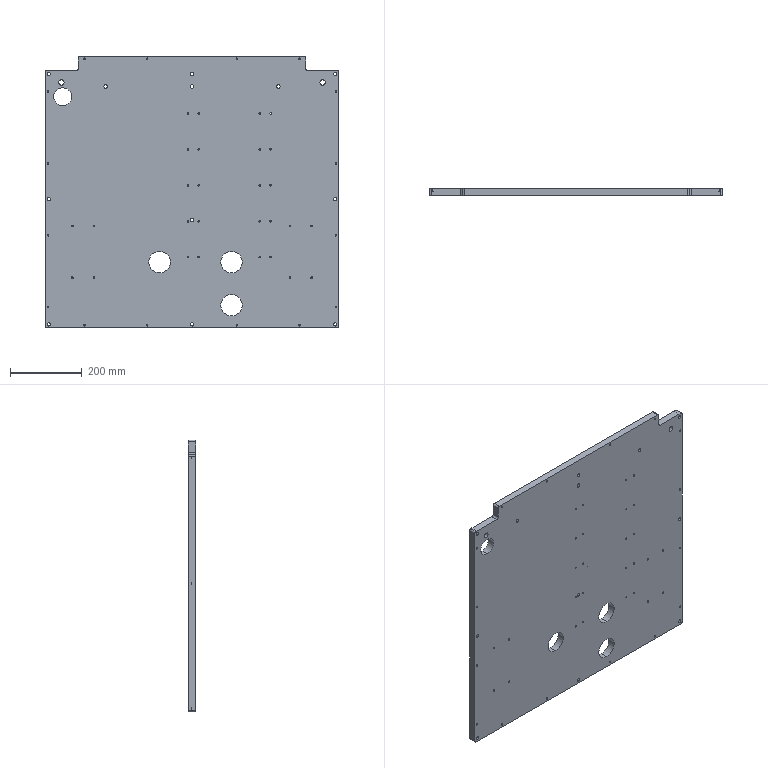Part | SolidWorks | features HoleWzd 10, ICE 5, LPattern 2, Extrusion 1, Fillet 1 | 1 solid | 285 faces | box 817 x 20 x 757 mm | volume 11961283 mm3 | cylinder 208 | cone 58 | plane 19 | commonest cylinder face diameters 4.2 x52 5 x48 2.5 x30 15 x22 9 x18 6 x16